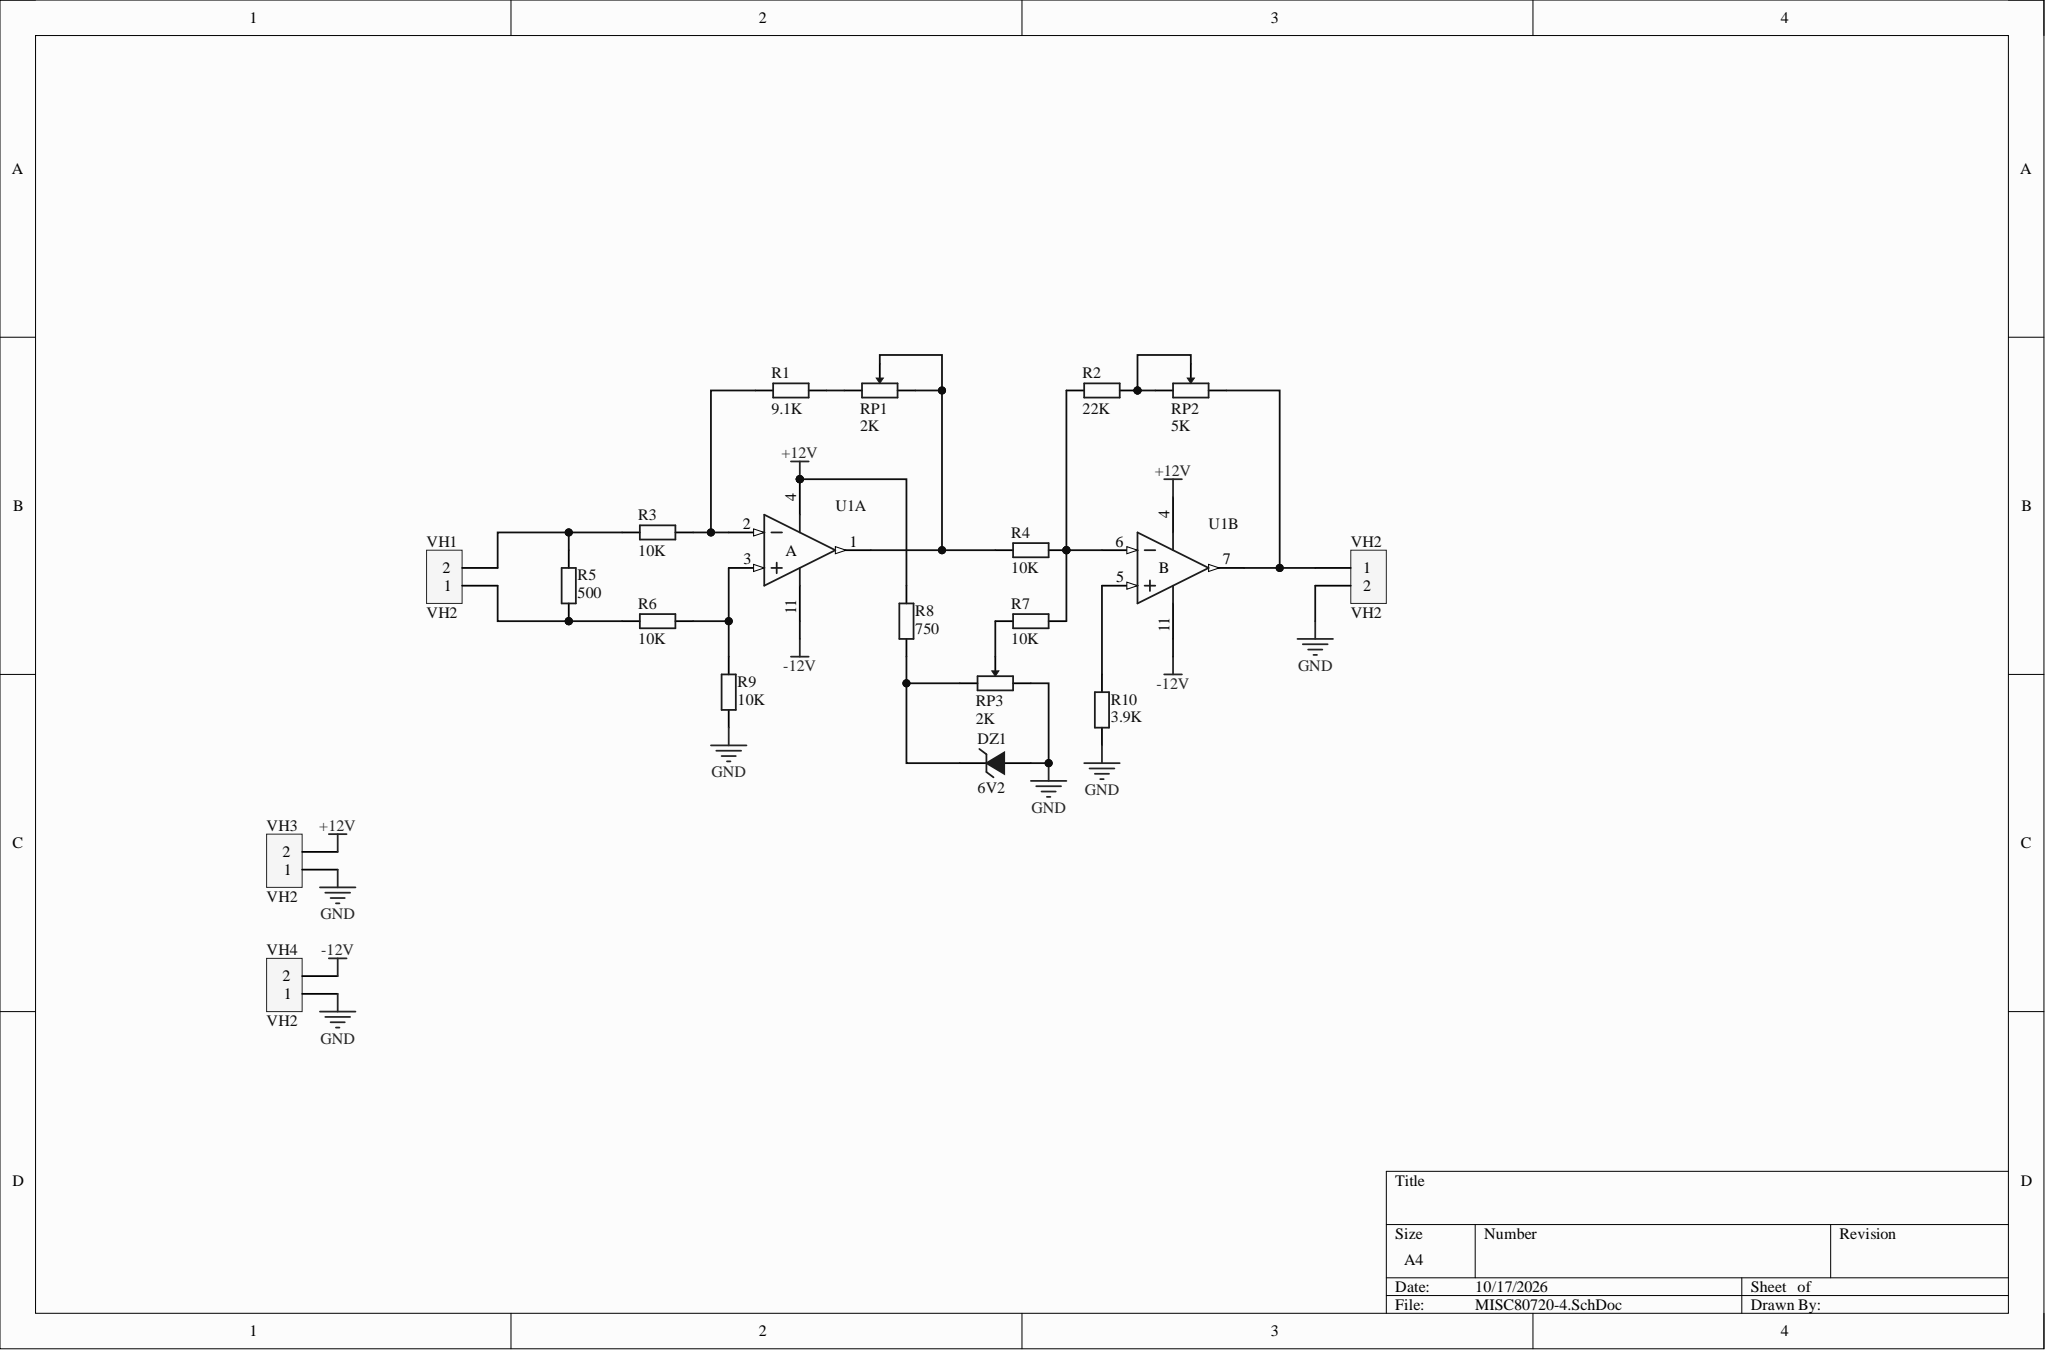Circuit board | Altium Designer | 19 parts | 15 nets
Bill of materials:
Comment,Description,Designator,Footprint,LibRef,Quantity
"6V2","12V/0.5W Zener diode","DZ1","DO-35","1N4106","1"
"9.1K","Color-band resistor","R1","RS 1/4W","R-S","1"
"22K","Color-band resistor","R2","RS 1/4W","R-S","1"
"10K","Color-band resistor","R3, R4, R6, R7, R9","RS 1/4W","R-S","5"
"500","Color-band resistor","R5","RS 1/4W","R-S","1"
"750","Color-band resistor","R8","RS 1/4W","R-S","1"
"3.9K","Color-band resistor","R10","RS 1/4W","R-S","1"
"2K","Single-gang potentiometer","RP1, RP3","3296W","RP","2"
"5K","Single-gang potentiometer","RP2","3296W","RP","1"
"LM124AD","Low-Power Quad Operational Amplifier","U1","DIP14","LM124AD","1"
"VH2","","VH1, VH2, VH3, VH4","VH3.96-2A","VH2","4"
Netlist (Protel format):
[
DZ1
DO-35
6V2



]
[
R1
RS 1/4W
9.1K



]
[
R2
RS 1/4W
22K



]
[
R3
RS 1/4W
10K



]
[
R4
RS 1/4W
10K



]
[
R5
RS 1/4W
500



]
[
R6
RS 1/4W
10K



]
[
R7
RS 1/4W
10K



]
[
R8
RS 1/4W
750



]
[
R9
RS 1/4W
10K



]
[
R10
RS 1/4W
3.9K



]
[
RP1
3296W
2K



]
[
RP2
3296W
5K



]
[
RP3
3296W
2K



]
[
U1
DIP14
LM124AD



]
[
VH1
VH3.96-2A
VH2



]
[
VH2
VH3.96-2A
VH2



]
[
VH3
VH3.96-2A
VH2



]
[
VH4
VH3.96-2A
VH2



]
(
NetRP2_3
RP2-3
U1-7
VH2-1
)
(
NetR10_2
R10-2
U1-5
)
(
NetR7_1
R7-1
RP3-2
)
(
NetR6_2
R6-2
R9-2
U1-3
)
(
NetR5_1
R5-1
R6-1
VH1-1
)
(
NetR4_1
R4-1
RP1-2
RP1-3
U1-1
)
(
NetR3_1
R3-1
R5-2
VH1-2
)
(
NetR2_2
R2-2
RP2-1
RP2-2
)
(
NetR2_1
R2-1
R4-2
R7-2
U1-6
)
(
NetR1_2
R1-2
RP1-1
)
(
NetR1_1
R1-1
R3-2
U1-2
)
(
NetDZ1_2
DZ1-2
R8-1
RP3-1
)
(
GND
DZ1-1
R9-1
R10-1
RP3-3
VH2-2
VH3-1
VH4-1
)
(
-12V
U1-11
VH4-2
)
(
+12V
R8-2
U1-4
VH3-2
)